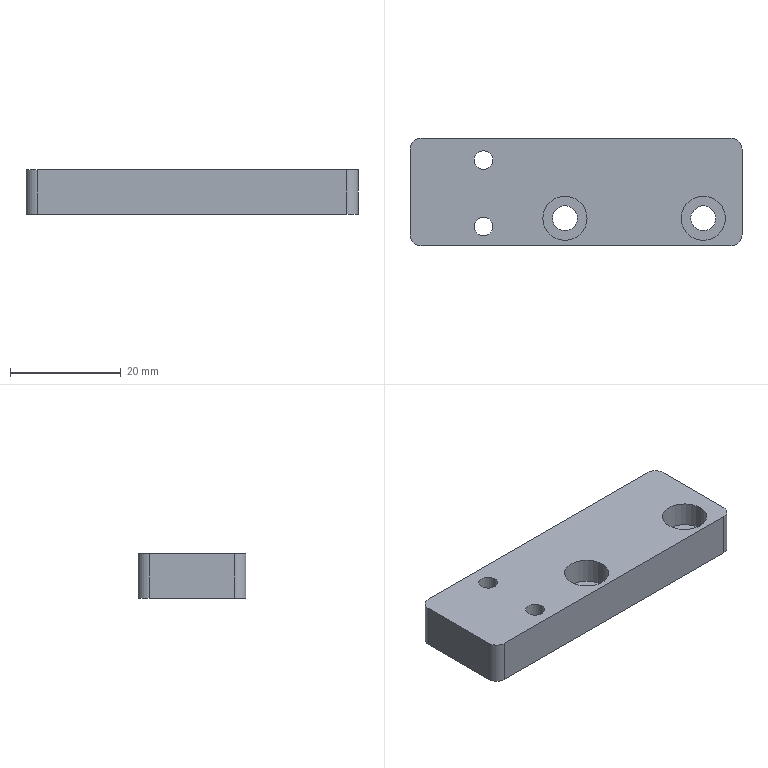Part | STEP file | FBDS-CS-001 | 1 solid | 30 faces | box 60 x 19.5 x 8 mm | volume 8486 mm3 | cylinder 20 | plane 10 | commonest cylinder face diameters 3.4 x4 4 x4 4.5 x4 6 x4 8 x4
STEP:
#1=CARTESIAN_POINT('',(16.3,15.5,3.4));
#2=VERTEX_POINT('',#1);
#3=CARTESIAN_POINT('',(10.3,15.5,3.4));
#4=VERTEX_POINT('',#3);
#5=CARTESIAN_POINT('',(13.3,15.5,3.4));
#6=DIRECTION('',(0.,0.,-1.));
#7=DIRECTION('',(-1.,0.,0.));
#8=AXIS2_PLACEMENT_3D('',#5,#6,#7);
#9=CIRCLE('',#8,3.);
#10=EDGE_CURVE('',#2,#4,#9,.T.);
#11=ORIENTED_EDGE('',*,*,#10,.F.);
#12=CARTESIAN_POINT('',(16.3,15.5,0.));
#13=VERTEX_POINT('',#12);
#14=CARTESIAN_POINT('',(16.3,15.5,0.));
#15=DIRECTION('',(0.,0.,-1.));
#16=VECTOR('',#15,1000.);
#17=LINE('',#14,#16);
#18=EDGE_CURVE('',#2,#13,#17,.T.);
#19=ORIENTED_EDGE('',*,*,#18,.T.);
#20=CARTESIAN_POINT('',(10.3,15.5,0.));
#21=VERTEX_POINT('',#20);
#22=CARTESIAN_POINT('',(13.3,15.5,0.));
#23=DIRECTION('',(0.,0.,-1.));
#24=DIRECTION('',(-1.,0.,0.));
#25=AXIS2_PLACEMENT_3D('',#22,#23,#24);
#26=CIRCLE('',#25,3.);
#27=EDGE_CURVE('',#13,#21,#26,.T.);
#28=ORIENTED_EDGE('',*,*,#27,.T.);
#29=CARTESIAN_POINT('',(10.3,15.5,0.));
#30=DIRECTION('',(0.,0.,-1.));
#31=VECTOR('',#30,1000.);
#32=LINE('',#29,#31);
#33=EDGE_CURVE('',#4,#21,#32,.T.);
#34=ORIENTED_EDGE('',*,*,#33,.F.);
#35=EDGE_LOOP('',(#11,#19,#28,#34));
#36=FACE_OUTER_BOUND('',#35,.T.);
#37=CARTESIAN_POINT('',(13.3,15.5,0.));
#38=DIRECTION('',(0.,0.,-1.));
#39=DIRECTION('',(-1.,0.,0.));
#40=AXIS2_PLACEMENT_3D('',#37,#38,#39);
#41=CYLINDRICAL_SURFACE('',#40,3.);
#42=ADVANCED_FACE('',(#36),#41,.F.);
#43=CARTESIAN_POINT('',(15.,15.5,8.));
#44=VERTEX_POINT('',#43);
#45=CARTESIAN_POINT('',(11.6,15.5,8.));
#46=VERTEX_POINT('',#45);
#47=CARTESIAN_POINT('',(13.3,15.5,8.));
#48=DIRECTION('',(0.,0.,-1.));
#49=DIRECTION('',(-1.,0.,0.));
#50=AXIS2_PLACEMENT_3D('',#47,#48,#49);
#51=CIRCLE('',#50,1.7);
#52=EDGE_CURVE('',#44,#46,#51,.T.);
#53=ORIENTED_EDGE('',*,*,#52,.F.);
#54=CARTESIAN_POINT('',(15.,15.5,3.4));
#55=VERTEX_POINT('',#54);
#56=CARTESIAN_POINT('',(15.,15.5,0.));
#57=DIRECTION('',(0.,0.,-1.));
#58=VECTOR('',#57,1000.);
#59=LINE('',#56,#58);
#60=EDGE_CURVE('',#44,#55,#59,.T.);
#61=ORIENTED_EDGE('',*,*,#60,.T.);
#62=CARTESIAN_POINT('',(11.6,15.5,3.4));
#63=VERTEX_POINT('',#62);
#64=CARTESIAN_POINT('',(13.3,15.5,3.4));
#65=DIRECTION('',(0.,0.,-1.));
#66=DIRECTION('',(-1.,0.,0.));
#67=AXIS2_PLACEMENT_3D('',#64,#65,#66);
#68=CIRCLE('',#67,1.7);
#69=EDGE_CURVE('',#55,#63,#68,.T.);
#70=ORIENTED_EDGE('',*,*,#69,.T.);
#71=CARTESIAN_POINT('',(11.6,15.5,0.));
#72=DIRECTION('',(0.,0.,-1.));
#73=VECTOR('',#72,1000.);
#74=LINE('',#71,#73);
#75=EDGE_CURVE('',#46,#63,#74,.T.);
#76=ORIENTED_EDGE('',*,*,#75,.F.);
#77=EDGE_LOOP('',(#53,#61,#70,#76));
#78=FACE_OUTER_BOUND('',#77,.T.);
#79=CARTESIAN_POINT('',(13.3,15.5,0.));
#80=DIRECTION('',(0.,0.,-1.));
#81=DIRECTION('',(-1.,0.,0.));
#82=AXIS2_PLACEMENT_3D('',#79,#80,#81);
#83=CYLINDRICAL_SURFACE('',#82,1.7);
#84=ADVANCED_FACE('',(#78),#83,.F.);
#85=CARTESIAN_POINT('',(16.3,3.5,3.4));
#86=VERTEX_POINT('',#85);
#87=CARTESIAN_POINT('',(10.3,3.5,3.4));
#88=VERTEX_POINT('',#87);
#89=CARTESIAN_POINT('',(13.3,3.5,3.4));
#90=DIRECTION('',(0.,0.,-1.));
#91=DIRECTION('',(-1.,0.,0.));
#92=AXIS2_PLACEMENT_3D('',#89,#90,#91);
#93=CIRCLE('',#92,3.);
#94=EDGE_CURVE('',#86,#88,#93,.T.);
#95=ORIENTED_EDGE('',*,*,#94,.F.);
#96=CARTESIAN_POINT('',(16.3,3.5,0.));
#97=VERTEX_POINT('',#96);
#98=CARTESIAN_POINT('',(16.3,3.5,0.));
#99=DIRECTION('',(0.,0.,-1.));
#100=VECTOR('',#99,1000.);
#101=LINE('',#98,#100);
#102=EDGE_CURVE('',#86,#97,#101,.T.);
#103=ORIENTED_EDGE('',*,*,#102,.T.);
#104=CARTESIAN_POINT('',(10.3,3.5,0.));
#105=VERTEX_POINT('',#104);
#106=CARTESIAN_POINT('',(13.3,3.5,0.));
#107=DIRECTION('',(0.,0.,-1.));
#108=DIRECTION('',(-1.,0.,0.));
#109=AXIS2_PLACEMENT_3D('',#106,#107,#108);
#110=CIRCLE('',#109,3.);
#111=EDGE_CURVE('',#97,#105,#110,.T.);
#112=ORIENTED_EDGE('',*,*,#111,.T.);
#113=CARTESIAN_POINT('',(10.3,3.5,0.));
#114=DIRECTION('',(0.,0.,-1.));
#115=VECTOR('',#114,1000.);
#116=LINE('',#113,#115);
#117=EDGE_CURVE('',#88,#105,#116,.T.);
#118=ORIENTED_EDGE('',*,*,#117,.F.);
#119=EDGE_LOOP('',(#95,#103,#112,#118));
#120=FACE_OUTER_BOUND('',#119,.T.);
#121=CARTESIAN_POINT('',(13.3,3.5,0.));
#122=DIRECTION('',(0.,0.,-1.));
#123=DIRECTION('',(-1.,0.,0.));
#124=AXIS2_PLACEMENT_3D('',#121,#122,#123);
#125=CYLINDRICAL_SURFACE('',#124,3.);
#126=ADVANCED_FACE('',(#120),#125,.F.);
#127=CARTESIAN_POINT('',(15.,3.5,8.));
#128=VERTEX_POINT('',#127);
#129=CARTESIAN_POINT('',(11.6,3.5,8.));
#130=VERTEX_POINT('',#129);
#131=CARTESIAN_POINT('',(13.3,3.5,8.));
#132=DIRECTION('',(0.,0.,-1.));
#133=DIRECTION('',(-1.,0.,0.));
#134=AXIS2_PLACEMENT_3D('',#131,#132,#133);
#135=CIRCLE('',#134,1.7);
#136=EDGE_CURVE('',#128,#130,#135,.T.);
#137=ORIENTED_EDGE('',*,*,#136,.F.);
#138=CARTESIAN_POINT('',(15.,3.5,3.4));
#139=VERTEX_POINT('',#138);
#140=CARTESIAN_POINT('',(15.,3.5,0.));
#141=DIRECTION('',(0.,0.,-1.));
#142=VECTOR('',#141,1000.);
#143=LINE('',#140,#142);
#144=EDGE_CURVE('',#128,#139,#143,.T.);
#145=ORIENTED_EDGE('',*,*,#144,.T.);
#146=CARTESIAN_POINT('',(11.6,3.5,3.4));
#147=VERTEX_POINT('',#146);
#148=CARTESIAN_POINT('',(13.3,3.5,3.4));
#149=DIRECTION('',(0.,0.,-1.));
#150=DIRECTION('',(-1.,0.,0.));
#151=AXIS2_PLACEMENT_3D('',#148,#149,#150);
#152=CIRCLE('',#151,1.7);
#153=EDGE_CURVE('',#139,#147,#152,.T.);
#154=ORIENTED_EDGE('',*,*,#153,.T.);
#155=CARTESIAN_POINT('',(11.6,3.5,0.));
#156=DIRECTION('',(0.,0.,-1.));
#157=VECTOR('',#156,1000.);
#158=LINE('',#155,#157);
#159=EDGE_CURVE('',#130,#147,#158,.T.);
#160=ORIENTED_EDGE('',*,*,#159,.F.);
#161=EDGE_LOOP('',(#137,#145,#154,#160));
#162=FACE_OUTER_BOUND('',#161,.T.);
#163=CARTESIAN_POINT('',(13.3,3.5,0.));
#164=DIRECTION('',(0.,0.,-1.));
#165=DIRECTION('',(-1.,0.,0.));
#166=AXIS2_PLACEMENT_3D('',#163,#164,#165);
#167=CYLINDRICAL_SURFACE('',#166,1.7);
#168=ADVANCED_FACE('',(#162),#167,.F.);
#169=CARTESIAN_POINT('',(24.,5.,3.4));
#170=VERTEX_POINT('',#169);
#171=CARTESIAN_POINT('',(32.,5.,3.4));
#172=VERTEX_POINT('',#171);
#173=CARTESIAN_POINT('',(28.,5.,3.4));
#174=DIRECTION('',(0.,0.,1.));
#175=DIRECTION('',(1.,0.,0.));
#176=AXIS2_PLACEMENT_3D('',#173,#174,#175);
#177=CIRCLE('',#176,4.);
#178=EDGE_CURVE('',#170,#172,#177,.T.);
#179=ORIENTED_EDGE('',*,*,#178,.F.);
#180=CARTESIAN_POINT('',(24.,5.,8.));
#181=VERTEX_POINT('',#180);
#182=CARTESIAN_POINT('',(24.,5.,8.));
#183=DIRECTION('',(0.,0.,1.));
#184=VECTOR('',#183,1000.);
#185=LINE('',#182,#184);
#186=EDGE_CURVE('',#170,#181,#185,.T.);
#187=ORIENTED_EDGE('',*,*,#186,.T.);
#188=CARTESIAN_POINT('',(32.,5.,8.));
#189=VERTEX_POINT('',#188);
#190=CARTESIAN_POINT('',(28.,5.,8.));
#191=DIRECTION('',(0.,0.,1.));
#192=DIRECTION('',(1.,0.,0.));
#193=AXIS2_PLACEMENT_3D('',#190,#191,#192);
#194=CIRCLE('',#193,4.);
#195=EDGE_CURVE('',#181,#189,#194,.T.);
#196=ORIENTED_EDGE('',*,*,#195,.T.);
#197=CARTESIAN_POINT('',(32.,5.,8.));
#198=DIRECTION('',(0.,0.,1.));
#199=VECTOR('',#198,1000.);
#200=LINE('',#197,#199);
#201=EDGE_CURVE('',#172,#189,#200,.T.);
#202=ORIENTED_EDGE('',*,*,#201,.F.);
#203=EDGE_LOOP('',(#179,#187,#196,#202));
#204=FACE_OUTER_BOUND('',#203,.T.);
#205=CARTESIAN_POINT('',(28.,5.,8.));
#206=DIRECTION('',(0.,0.,1.));
#207=DIRECTION('',(1.,0.,0.));
#208=AXIS2_PLACEMENT_3D('',#205,#206,#207);
#209=CYLINDRICAL_SURFACE('',#208,4.);
#210=ADVANCED_FACE('',(#204),#209,.F.);
#211=CARTESIAN_POINT('',(25.75,5.,0.));
#212=VERTEX_POINT('',#211);
#213=CARTESIAN_POINT('',(30.25,5.,0.));
#214=VERTEX_POINT('',#213);
#215=CARTESIAN_POINT('',(28.,5.,0.));
#216=DIRECTION('',(0.,0.,1.));
#217=DIRECTION('',(1.,0.,0.));
#218=AXIS2_PLACEMENT_3D('',#215,#216,#217);
#219=CIRCLE('',#218,2.25);
#220=EDGE_CURVE('',#212,#214,#219,.T.);
#221=ORIENTED_EDGE('',*,*,#220,.F.);
#222=CARTESIAN_POINT('',(25.75,5.,3.4));
#223=VERTEX_POINT('',#222);
#224=CARTESIAN_POINT('',(25.75,5.,8.));
#225=DIRECTION('',(0.,0.,1.));
#226=VECTOR('',#225,1000.);
#227=LINE('',#224,#226);
#228=EDGE_CURVE('',#212,#223,#227,.T.);
#229=ORIENTED_EDGE('',*,*,#228,.T.);
#230=CARTESIAN_POINT('',(30.25,5.,3.4));
#231=VERTEX_POINT('',#230);
#232=CARTESIAN_POINT('',(28.,5.,3.4));
#233=DIRECTION('',(0.,0.,1.));
#234=DIRECTION('',(1.,0.,0.));
#235=AXIS2_PLACEMENT_3D('',#232,#233,#234);
#236=CIRCLE('',#235,2.25);
#237=EDGE_CURVE('',#223,#231,#236,.T.);
#238=ORIENTED_EDGE('',*,*,#237,.T.);
#239=CARTESIAN_POINT('',(30.25,5.,8.));
#240=DIRECTION('',(0.,0.,1.));
#241=VECTOR('',#240,1000.);
#242=LINE('',#239,#241);
#243=EDGE_CURVE('',#214,#231,#242,.T.);
#244=ORIENTED_EDGE('',*,*,#243,.F.);
#245=EDGE_LOOP('',(#221,#229,#238,#244));
#246=FACE_OUTER_BOUND('',#245,.T.);
#247=CARTESIAN_POINT('',(28.,5.,8.));
#248=DIRECTION('',(0.,0.,1.));
#249=DIRECTION('',(1.,0.,0.));
#250=AXIS2_PLACEMENT_3D('',#247,#248,#249);
#251=CYLINDRICAL_SURFACE('',#250,2.25);
#252=ADVANCED_FACE('',(#246),#251,.F.);
#253=CARTESIAN_POINT('',(49.,5.,3.4));
#254=VERTEX_POINT('',#253);
#255=CARTESIAN_POINT('',(57.,5.,3.4));
#256=VERTEX_POINT('',#255);
#257=CARTESIAN_POINT('',(53.,5.,3.4));
#258=DIRECTION('',(0.,0.,1.));
#259=DIRECTION('',(1.,0.,0.));
#260=AXIS2_PLACEMENT_3D('',#257,#258,#259);
#261=CIRCLE('',#260,4.);
#262=EDGE_CURVE('',#254,#256,#261,.T.);
#263=ORIENTED_EDGE('',*,*,#262,.F.);
#264=CARTESIAN_POINT('',(49.,5.,8.));
#265=VERTEX_POINT('',#264);
#266=CARTESIAN_POINT('',(49.,5.,8.));
#267=DIRECTION('',(0.,0.,1.));
#268=VECTOR('',#267,1000.);
#269=LINE('',#266,#268);
#270=EDGE_CURVE('',#254,#265,#269,.T.);
#271=ORIENTED_EDGE('',*,*,#270,.T.);
#272=CARTESIAN_POINT('',(57.,5.,8.));
#273=VERTEX_POINT('',#272);
#274=CARTESIAN_POINT('',(53.,5.,8.));
#275=DIRECTION('',(0.,0.,1.));
#276=DIRECTION('',(1.,0.,0.));
#277=AXIS2_PLACEMENT_3D('',#274,#275,#276);
#278=CIRCLE('',#277,4.);
#279=EDGE_CURVE('',#265,#273,#278,.T.);
#280=ORIENTED_EDGE('',*,*,#279,.T.);
#281=CARTESIAN_POINT('',(57.,5.,8.));
#282=DIRECTION('',(0.,0.,1.));
#283=VECTOR('',#282,1000.);
#284=LINE('',#281,#283);
#285=EDGE_CURVE('',#256,#273,#284,.T.);
#286=ORIENTED_EDGE('',*,*,#285,.F.);
#287=EDGE_LOOP('',(#263,#271,#280,#286));
#288=FACE_OUTER_BOUND('',#287,.T.);
#289=CARTESIAN_POINT('',(53.,5.,8.));
#290=DIRECTION('',(0.,0.,1.));
#291=DIRECTION('',(1.,0.,0.));
#292=AXIS2_PLACEMENT_3D('',#289,#290,#291);
#293=CYLINDRICAL_SURFACE('',#292,4.);
#294=ADVANCED_FACE('',(#288),#293,.F.);
#295=CARTESIAN_POINT('',(50.75,5.,0.));
#296=VERTEX_POINT('',#295);
#297=CARTESIAN_POINT('',(55.25,5.,0.));
#298=VERTEX_POINT('',#297);
#299=CARTESIAN_POINT('',(53.,5.,0.));
#300=DIRECTION('',(0.,0.,1.));
#301=DIRECTION('',(1.,0.,0.));
#302=AXIS2_PLACEMENT_3D('',#299,#300,#301);
#303=CIRCLE('',#302,2.25);
#304=EDGE_CURVE('',#296,#298,#303,.T.);
#305=ORIENTED_EDGE('',*,*,#304,.F.);
#306=CARTESIAN_POINT('',(50.75,5.,3.4));
#307=VERTEX_POINT('',#306);
#308=CARTESIAN_POINT('',(50.75,5.,8.));
#309=DIRECTION('',(0.,0.,1.));
#310=VECTOR('',#309,1000.);
#311=LINE('',#308,#310);
#312=EDGE_CURVE('',#296,#307,#311,.T.);
#313=ORIENTED_EDGE('',*,*,#312,.T.);
#314=CARTESIAN_POINT('',(55.25,5.,3.4));
#315=VERTEX_POINT('',#314);
#316=CARTESIAN_POINT('',(53.,5.,3.4));
#317=DIRECTION('',(0.,0.,1.));
#318=DIRECTION('',(1.,0.,0.));
#319=AXIS2_PLACEMENT_3D('',#316,#317,#318);
#320=CIRCLE('',#319,2.25);
#321=EDGE_CURVE('',#307,#315,#320,.T.);
#322=ORIENTED_EDGE('',*,*,#321,.T.);
#323=CARTESIAN_POINT('',(55.25,5.,8.));
#324=DIRECTION('',(0.,0.,1.));
#325=VECTOR('',#324,1000.);
#326=LINE('',#323,#325);
#327=EDGE_CURVE('',#298,#315,#326,.T.);
#328=ORIENTED_EDGE('',*,*,#327,.F.);
#329=EDGE_LOOP('',(#305,#313,#322,#328));
#330=FACE_OUTER_BOUND('',#329,.T.);
#331=CARTESIAN_POINT('',(53.,5.,8.));
#332=DIRECTION('',(0.,0.,1.));
#333=DIRECTION('',(1.,0.,0.));
#334=AXIS2_PLACEMENT_3D('',#331,#332,#333);
#335=CYLINDRICAL_SURFACE('',#334,2.25);
#336=ADVANCED_FACE('',(#330),#335,.F.);
#337=CARTESIAN_POINT('',(0.,17.5,0.));
#338=VERTEX_POINT('',#337);
#339=CARTESIAN_POINT('',(0.,2.,0.));
#340=VERTEX_POINT('',#339);
#341=CARTESIAN_POINT('',(0.,0.,0.));
#342=DIRECTION('',(0.,-1.,0.));
#343=VECTOR('',#342,1000.);
#344=LINE('',#341,#343);
#345=EDGE_CURVE('',#338,#340,#344,.T.);
#346=ORIENTED_EDGE('',*,*,#345,.T.);
#347=CARTESIAN_POINT('',(0.,2.,8.));
#348=VERTEX_POINT('',#347);
#349=CARTESIAN_POINT('',(0.,2.,8.));
#350=DIRECTION('',(0.,0.,1.));
#351=VECTOR('',#350,1000.);
#352=LINE('',#349,#351);
#353=EDGE_CURVE('',#340,#348,#352,.T.);
#354=ORIENTED_EDGE('',*,*,#353,.T.);
#355=CARTESIAN_POINT('',(0.,17.5,8.));
#356=VERTEX_POINT('',#355);
#357=CARTESIAN_POINT('',(0.,0.,8.));
#358=DIRECTION('',(0.,-1.,0.));
#359=VECTOR('',#358,1000.);
#360=LINE('',#357,#359);
#361=EDGE_CURVE('',#356,#348,#360,.T.);
#362=ORIENTED_EDGE('',*,*,#361,.F.);
#363=CARTESIAN_POINT('',(0.,17.5,8.));
#364=DIRECTION('',(0.,0.,-1.));
#365=VECTOR('',#364,1000.);
#366=LINE('',#363,#365);
#367=EDGE_CURVE('',#356,#338,#366,.T.);
#368=ORIENTED_EDGE('',*,*,#367,.T.);
#369=EDGE_LOOP('',(#346,#354,#362,#368));
#370=FACE_OUTER_BOUND('',#369,.T.);
#371=CARTESIAN_POINT('',(0.,0.,8.));
#372=DIRECTION('',(1.,0.,0.));
#373=DIRECTION('',(0.,0.,-1.));
#374=AXIS2_PLACEMENT_3D('',#371,#372,#373);
#375=PLANE('',#374);
#376=ADVANCED_FACE('',(#370),#375,.F.);
#377=CARTESIAN_POINT('',(2.,0.,0.));
#378=VERTEX_POINT('',#377);
#379=CARTESIAN_POINT('',(58.,0.,0.));
#380=VERTEX_POINT('',#379);
#381=CARTESIAN_POINT('',(0.,0.,0.));
#382=DIRECTION('',(1.,0.,0.));
#383=VECTOR('',#382,1000.);
#384=LINE('',#381,#383);
#385=EDGE_CURVE('',#378,#380,#384,.T.);
#386=ORIENTED_EDGE('',*,*,#385,.T.);
#387=CARTESIAN_POINT('',(58.,0.,8.));
#388=VERTEX_POINT('',#387);
#389=CARTESIAN_POINT('',(58.,0.,8.));
#390=DIRECTION('',(0.,0.,1.));
#391=VECTOR('',#390,1000.);
#392=LINE('',#389,#391);
#393=EDGE_CURVE('',#380,#388,#392,.T.);
#394=ORIENTED_EDGE('',*,*,#393,.T.);
#395=CARTESIAN_POINT('',(2.,0.,8.));
#396=VERTEX_POINT('',#395);
#397=CARTESIAN_POINT('',(0.,0.,8.));
#398=DIRECTION('',(1.,0.,0.));
#399=VECTOR('',#398,1000.);
#400=LINE('',#397,#399);
#401=EDGE_CURVE('',#396,#388,#400,.T.);
#402=ORIENTED_EDGE('',*,*,#401,.F.);
#403=CARTESIAN_POINT('',(2.,0.,8.));
#404=DIRECTION('',(0.,0.,-1.));
#405=VECTOR('',#404,1000.);
#406=LINE('',#403,#405);
#407=EDGE_CURVE('',#396,#378,#406,.T.);
#408=ORIENTED_EDGE('',*,*,#407,.T.);
#409=EDGE_LOOP('',(#386,#394,#402,#408));
#410=FACE_OUTER_BOUND('',#409,.T.);
#411=CARTESIAN_POINT('',(0.,0.,8.));
#412=DIRECTION('',(0.,1.,0.));
#413=DIRECTION('',(0.,0.,1.));
#414=AXIS2_PLACEMENT_3D('',#411,#412,#413);
#415=PLANE('',#414);
#416=ADVANCED_FACE('',(#410),#415,.F.);
#417=CARTESIAN_POINT('',(60.,2.,8.));
#418=VERTEX_POINT('',#417);
#419=CARTESIAN_POINT('',(60.,17.5,8.));
#420=VERTEX_POINT('',#419);
#421=CARTESIAN_POINT('',(60.,0.,8.));
#422=DIRECTION('',(0.,1.,0.));
#423=VECTOR('',#422,1000.);
#424=LINE('',#421,#423);
#425=EDGE_CURVE('',#418,#420,#424,.T.);
#426=ORIENTED_EDGE('',*,*,#425,.F.);
#427=CARTESIAN_POINT('',(60.,2.,0.));
#428=VERTEX_POINT('',#427);
#429=CARTESIAN_POINT('',(60.,2.,8.));
#430=DIRECTION('',(0.,0.,-1.));
#431=VECTOR('',#430,1000.);
#432=LINE('',#429,#431);
#433=EDGE_CURVE('',#418,#428,#432,.T.);
#434=ORIENTED_EDGE('',*,*,#433,.T.);
#435=CARTESIAN_POINT('',(60.,17.5,0.));
#436=VERTEX_POINT('',#435);
#437=CARTESIAN_POINT('',(60.,0.,0.));
#438=DIRECTION('',(0.,1.,0.));
#439=VECTOR('',#438,1000.);
#440=LINE('',#437,#439);
#441=EDGE_CURVE('',#428,#436,#440,.T.);
#442=ORIENTED_EDGE('',*,*,#441,.T.);
#443=CARTESIAN_POINT('',(60.,17.5,8.));
#444=DIRECTION('',(0.,0.,1.));
#445=VECTOR('',#444,1000.);
#446=LINE('',#443,#445);
#447=EDGE_CURVE('',#436,#420,#446,.T.);
#448=ORIENTED_EDGE('',*,*,#447,.T.);
#449=EDGE_LOOP('',(#426,#434,#442,#448));
#450=FACE_OUTER_BOUND('',#449,.T.);
#451=CARTESIAN_POINT('',(60.,0.,8.));
#452=DIRECTION('',(-1.,0.,0.));
#453=DIRECTION('',(0.,0.,1.));
#454=AXIS2_PLACEMENT_3D('',#451,#452,#453);
#455=PLANE('',#454);
#456=ADVANCED_FACE('',(#450),#455,.F.);
#457=CARTESIAN_POINT('',(58.,19.5,8.));
#458=VERTEX_POINT('',#457);
#459=CARTESIAN_POINT('',(2.,19.5,8.));
#460=VERTEX_POINT('',#459);
#461=CARTESIAN_POINT('',(0.,19.5,8.));
#462=DIRECTION('',(-1.,0.,0.));
#463=VECTOR('',#462,1000.);
#464=LINE('',#461,#463);
#465=EDGE_CURVE('',#458,#460,#464,.T.);
#466=ORIENTED_EDGE('',*,*,#465,.F.);
#467=CARTESIAN_POINT('',(58.,19.5,0.));
#468=VERTEX_POINT('',#467);
#469=CARTESIAN_POINT('',(58.,19.5,8.));
#470=DIRECTION('',(0.,0.,-1.));
#471=VECTOR('',#470,1000.);
#472=LINE('',#469,#471);
#473=EDGE_CURVE('',#458,#468,#472,.T.);
#474=ORIENTED_EDGE('',*,*,#473,.T.);
#475=CARTESIAN_POINT('',(2.,19.5,0.));
#476=VERTEX_POINT('',#475);
#477=CARTESIAN_POINT('',(0.,19.5,0.));
#478=DIRECTION('',(-1.,0.,0.));
#479=VECTOR('',#478,1000.);
#480=LINE('',#477,#479);
#481=EDGE_CURVE('',#468,#476,#480,.T.);
#482=ORIENTED_EDGE('',*,*,#481,.T.);
#483=CARTESIAN_POINT('',(2.,19.5,8.));
#484=DIRECTION('',(0.,0.,1.));
#485=VECTOR('',#484,1000.);
#486=LINE('',#483,#485);
#487=EDGE_CURVE('',#476,#460,#486,.T.);
#488=ORIENTED_EDGE('',*,*,#487,.T.);
#489=EDGE_LOOP('',(#466,#474,#482,#488));
#490=FACE_OUTER_BOUND('',#489,.T.);
#491=CARTESIAN_POINT('',(0.,19.5,8.));
#492=DIRECTION('',(0.,-1.,0.));
#493=DIRECTION('',(0.,0.,-1.));
#494=AXIS2_PLACEMENT_3D('',#491,#492,#493);
#495=PLANE('',#494);
#496=ADVANCED_FACE('',(#490),#495,.F.);
#497=CARTESIAN_POINT('',(13.3,15.5,8.));
#498=DIRECTION('',(0.,0.,-1.));
#499=DIRECTION('',(-1.,0.,0.));
#500=AXIS2_PLACEMENT_3D('',#497,#498,#499);
#501=CIRCLE('',#500,1.7);
#502=EDGE_CURVE('',#46,#44,#501,.T.);
#503=ORIENTED_EDGE('',*,*,#502,.T.);
#504=ORIENTED_EDGE('',*,*,#52,.T.);
#505=EDGE_LOOP('',(#503,#504));
#506=FACE_BOUND('',#505,.T.);
#507=CARTESIAN_POINT('',(13.3,3.5,8.));
#508=DIRECTION('',(0.,0.,-1.));
#509=DIRECTION('',(-1.,0.,0.));
#510=AXIS2_PLACEMENT_3D('',#507,#508,#509);
#511=CIRCLE('',#510,1.7);
#512=EDGE_CURVE('',#130,#128,#511,.T.);
#513=ORIENTED_EDGE('',*,*,#512,.T.);
#514=ORIENTED_EDGE('',*,*,#136,.T.);
#515=EDGE_LOOP('',(#513,#514));
#516=FACE_BOUND('',#515,.T.);
#517=CARTESIAN_POINT('',(28.,5.,8.));
#518=DIRECTION('',(0.,0.,1.));
#519=DIRECTION('',(1.,0.,0.));
#520=AXIS2_PLACEMENT_3D('',#517,#518,#519);
#521=CIRCLE('',#520,4.);
#522=EDGE_CURVE('',#189,#181,#521,.T.);
#523=ORIENTED_EDGE('',*,*,#522,.F.);
#524=ORIENTED_EDGE('',*,*,#195,.F.);
#525=EDGE_LOOP('',(#523,#524));
#526=FACE_BOUND('',#525,.T.);
#527=CARTESIAN_POINT('',(53.,5.,8.));
#528=DIRECTION('',(0.,0.,1.));
#529=DIRECTION('',(1.,0.,0.));
#530=AXIS2_PLACEMENT_3D('',#527,#528,#529);
#531=CIRCLE('',#530,4.);
#532=EDGE_CURVE('',#273,#265,#531,.T.);
#533=ORIENTED_EDGE('',*,*,#532,.F.);
#534=ORIENTED_EDGE('',*,*,#279,.F.);
#535=EDGE_LOOP('',(#533,#534));
#536=FACE_BOUND('',#535,.T.);
#537=ORIENTED_EDGE('',*,*,#401,.T.);
#538=CARTESIAN_POINT('',(58.,2.,8.));
#539=DIRECTION('',(0.,0.,1.));
#540=DIRECTION('',(-1.,0.,0.));
#541=AXIS2_PLACEMENT_3D('',#538,#539,#540);
#542=CIRCLE('',#541,2.);
#543=EDGE_CURVE('',#388,#418,#542,.T.);
#544=ORIENTED_EDGE('',*,*,#543,.T.);
#545=ORIENTED_EDGE('',*,*,#425,.T.);
#546=CARTESIAN_POINT('',(58.,17.5,8.));
#547=DIRECTION('',(0.,0.,1.));
#548=DIRECTION('',(-1.,0.,0.));
#549=AXIS2_PLACEMENT_3D('',#546,#547,#548);
#550=CIRCLE('',#549,2.);
#551=EDGE_CURVE('',#420,#458,#550,.T.);
#552=ORIENTED_EDGE('',*,*,#551,.T.);
#553=ORIENTED_EDGE('',*,*,#465,.T.);
#554=CARTESIAN_POINT('',(2.,17.5,8.));
#555=DIRECTION('',(0.,0.,1.));
#556=DIRECTION('',(-1.,0.,0.));
#557=AXIS2_PLACEMENT_3D('',#554,#555,#556);
#558=CIRCLE('',#557,2.);
#559=EDGE_CURVE('',#460,#356,#558,.T.);
#560=ORIENTED_EDGE('',*,*,#559,.T.);
#561=ORIENTED_EDGE('',*,*,#361,.T.);
#562=CARTESIAN_POINT('',(2.,2.,8.));
#563=DIRECTION('',(0.,0.,1.));
#564=DIRECTION('',(-1.,0.,0.));
#565=AXIS2_PLACEMENT_3D('',#562,#563,#564);
#566=CIRCLE('',#565,2.);
#567=EDGE_CURVE('',#348,#396,#566,.T.);
#568=ORIENTED_EDGE('',*,*,#567,.T.);
#569=EDGE_LOOP('',(#537,#544,#545,#552,#553,#560,#561,#568));
#570=FACE_OUTER_BOUND('',#569,.T.);
#571=CARTESIAN_POINT('',(0.,0.,8.));
#572=DIRECTION('',(0.,0.,-1.));
#573=DIRECTION('',(-1.,0.,0.));
#574=AXIS2_PLACEMENT_3D('',#571,#572,#573);
#575=PLANE('',#574);
#576=ADVANCED_FACE('',(#506,#516,#526,#536,#570),#575,.F.);
#577=CARTESIAN_POINT('',(13.3,15.5,0.));
#578=DIRECTION('',(0.,0.,-1.));
#579=DIRECTION('',(-1.,0.,0.));
#580=AXIS2_PLACEMENT_3D('',#577,#578,#579);
#581=CIRCLE('',#580,3.);
#582=EDGE_CURVE('',#21,#13,#581,.T.);
#583=ORIENTED_EDGE('',*,*,#582,.F.);
#584=ORIENTED_EDGE('',*,*,#27,.F.);
#585=EDGE_LOOP('',(#583,#584));
#586=FACE_BOUND('',#585,.T.);
#587=CARTESIAN_POINT('',(13.3,3.5,0.));
#588=DIRECTION('',(0.,0.,-1.));
#589=DIRECTION('',(-1.,0.,0.));
#590=AXIS2_PLACEMENT_3D('',#587,#588,#589);
#591=CIRCLE('',#590,3.);
#592=EDGE_CURVE('',#105,#97,#591,.T.);
#593=ORIENTED_EDGE('',*,*,#592,.F.);
#594=ORIENTED_EDGE('',*,*,#111,.F.);
#595=EDGE_LOOP('',(#593,#594));
#596=FACE_BOUND('',#595,.T.);
#597=CARTESIAN_POINT('',(28.,5.,0.));
#598=DIRECTION('',(0.,0.,1.));
#599=DIRECTION('',(1.,0.,0.));
#600=AXIS2_PLACEMENT_3D('',#597,#598,#599);
#601=CIRCLE('',#600,2.25);
#602=EDGE_CURVE('',#214,#212,#601,.T.);
#603=ORIENTED_EDGE('',*,*,#602,.T.);
#604=ORIENTED_EDGE('',*,*,#220,.T.);
#605=EDGE_LOOP('',(#603,#604));
#606=FACE_BOUND('',#605,.T.);
#607=CARTESIAN_POINT('',(53.,5.,0.));
#608=DIRECTION('',(0.,0.,1.));
#609=DIRECTION('',(1.,0.,0.));
#610=AXIS2_PLACEMENT_3D('',#607,#608,#609);
#611=CIRCLE('',#610,2.25);
#612=EDGE_CURVE('',#298,#296,#611,.T.);
#613=ORIENTED_EDGE('',*,*,#612,.T.);
#614=ORIENTED_EDGE('',*,*,#304,.T.);
#615=EDGE_LOOP('',(#613,#614));
#616=FACE_BOUND('',#615,.T.);
#617=ORIENTED_EDGE('',*,*,#441,.F.);
#618=CARTESIAN_POINT('',(58.,2.,0.));
#619=DIRECTION('',(0.,0.,-1.));
#620=DIRECTION('',(-1.,0.,0.));
#621=AXIS2_PLACEMENT_3D('',#618,#619,#620);
#622=CIRCLE('',#621,2.);
#623=EDGE_CURVE('',#428,#380,#622,.T.);
#624=ORIENTED_EDGE('',*,*,#623,.T.);
#625=ORIENTED_EDGE('',*,*,#385,.F.);
#626=CARTESIAN_POINT('',(2.,2.,0.));
#627=DIRECTION('',(0.,0.,-1.));
#628=DIRECTION('',(-1.,0.,0.));
#629=AXIS2_PLACEMENT_3D('',#626,#627,#628);
#630=CIRCLE('',#629,2.);
#631=EDGE_CURVE('',#378,#340,#630,.T.);
#632=ORIENTED_EDGE('',*,*,#631,.T.);
#633=ORIENTED_EDGE('',*,*,#345,.F.);
#634=CARTESIAN_POINT('',(2.,17.5,0.));
#635=DIRECTION('',(0.,0.,-1.));
#636=DIRECTION('',(-1.,0.,0.));
#637=AXIS2_PLACEMENT_3D('',#634,#635,#636);
#638=CIRCLE('',#637,2.);
#639=EDGE_CURVE('',#338,#476,#638,.T.);
#640=ORIENTED_EDGE('',*,*,#639,.T.);
#641=ORIENTED_EDGE('',*,*,#481,.F.);
#642=CARTESIAN_POINT('',(58.,17.5,0.));
#643=DIRECTION('',(0.,0.,-1.));
#644=DIRECTION('',(-1.,0.,0.));
#645=AXIS2_PLACEMENT_3D('',#642,#643,#644);
#646=CIRCLE('',#645,2.);
#647=EDGE_CURVE('',#468,#436,#646,.T.);
#648=ORIENTED_EDGE('',*,*,#647,.T.);
#649=EDGE_LOOP('',(#617,#624,#625,#632,#633,#640,#641,#648));
#650=FACE_OUTER_BOUND('',#649,.T.);
#651=CARTESIAN_POINT('',(0.,0.,0.));
#652=DIRECTION('',(0.,0.,-1.));
#653=DIRECTION('',(-1.,0.,0.));
#654=AXIS2_PLACEMENT_3D('',#651,#652,#653);
#655=PLANE('',#654);
#656=ADVANCED_FACE('',(#586,#596,#606,#616,#650),#655,.T.);
#657=ORIENTED_EDGE('',*,*,#312,.F.);
#658=ORIENTED_EDGE('',*,*,#612,.F.);
#659=ORIENTED_EDGE('',*,*,#327,.T.);
#660=CARTESIAN_POINT('',(53.,5.,3.4));
#661=DIRECTION('',(0.,0.,1.));
#662=DIRECTION('',(1.,0.,0.));
#663=AXIS2_PLACEMENT_3D('',#660,#661,#662);
#664=CIRCLE('',#663,2.25);
#665=EDGE_CURVE('',#315,#307,#664,.T.);
#666=ORIENTED_EDGE('',*,*,#665,.T.);
#667=EDGE_LOOP('',(#657,#658,#659,#666));
#668=FACE_OUTER_BOUND('',#667,.T.);
#669=CARTESIAN_POINT('',(53.,5.,8.));
#670=DIRECTION('',(0.,0.,1.));
#671=DIRECTION('',(1.,0.,0.));
#672=AXIS2_PLACEMENT_3D('',#669,#670,#671);
#673=CYLINDRICAL_SURFACE('',#672,2.25);
#674=ADVANCED_FACE('',(#668),#673,.F.);
#675=ORIENTED_EDGE('',*,*,#665,.F.);
#676=ORIENTED_EDGE('',*,*,#321,.F.);
#677=EDGE_LOOP('',(#675,#676));
#678=FACE_BOUND('',#677,.T.);
#679=CARTESIAN_POINT('',(53.,5.,3.4));
#680=DIRECTION('',(0.,0.,1.));
#681=DIRECTION('',(1.,0.,0.));
#682=AXIS2_PLACEMENT_3D('',#679,#680,#681);
#683=CIRCLE('',#682,4.);
#684=EDGE_CURVE('',#256,#254,#683,.T.);
#685=ORIENTED_EDGE('',*,*,#684,.T.);
#686=ORIENTED_EDGE('',*,*,#262,.T.);
#687=EDGE_LOOP('',(#685,#686));
#688=FACE_OUTER_BOUND('',#687,.T.);
#689=CARTESIAN_POINT('',(55.25,5.,3.4));
#690=DIRECTION('',(0.,0.,-1.));
#691=DIRECTION('',(-1.,0.,0.));
#692=AXIS2_PLACEMENT_3D('',#689,#690,#691);
#693=PLANE('',#692);
#694=ADVANCED_FACE('',(#678,#688),#693,.F.);
#695=ORIENTED_EDGE('',*,*,#270,.F.);
#696=ORIENTED_EDGE('',*,*,#684,.F.);
#697=ORIENTED_EDGE('',*,*,#285,.T.);
#698=ORIENTED_EDGE('',*,*,#532,.T.);
#699=EDGE_LOOP('',(#695,#696,#697,#698));
#700=FACE_OUTER_BOUND('',#699,.T.);
#701=CARTESIAN_POINT('',(53.,5.,8.));
#702=DIRECTION('',(0.,0.,1.));
#703=DIRECTION('',(1.,0.,0.));
#704=AXIS2_PLACEMENT_3D('',#701,#702,#703);
#705=CYLINDRICAL_SURFACE('',#704,4.);
#706=ADVANCED_FACE('',(#700),#705,.F.);
#707=ORIENTED_EDGE('',*,*,#228,.F.);
#708=ORIENTED_EDGE('',*,*,#602,.F.);
#709=ORIENTED_EDGE('',*,*,#243,.T.);
#710=CARTESIAN_POINT('',(28.,5.,3.4));
#711=DIRECTION('',(0.,0.,1.));
#712=DIRECTION('',(1.,0.,0.));
#713=AXIS2_PLACEMENT_3D('',#710,#711,#712);
#714=CIRCLE('',#713,2.25);
#715=EDGE_CURVE('',#231,#223,#714,.T.);
#716=ORIENTED_EDGE('',*,*,#715,.T.);
#717=EDGE_LOOP('',(#707,#708,#709,#716));
#718=FACE_OUTER_BOUND('',#717,.T.);
#719=CARTESIAN_POINT('',(28.,5.,8.));
#720=DIRECTION('',(0.,0.,1.));
#721=DIRECTION('',(1.,0.,0.));
#722=AXIS2_PLACEMENT_3D('',#719,#720,#721);
#723=CYLINDRICAL_SURFACE('',#722,2.25);
#724=ADVANCED_FACE('',(#718),#723,.F.);
#725=ORIENTED_EDGE('',*,*,#715,.F.);
#726=ORIENTED_EDGE('',*,*,#237,.F.);
#727=EDGE_LOOP('',(#725,#726));
#728=FACE_BOUND('',#727,.T.);
#729=CARTESIAN_POINT('',(28.,5.,3.4));
#730=DIRECTION('',(0.,0.,1.));
#731=DIRECTION('',(1.,0.,0.));
#732=AXIS2_PLACEMENT_3D('',#729,#730,#731);
#733=CIRCLE('',#732,4.);
#734=EDGE_CURVE('',#172,#170,#733,.T.);
#735=ORIENTED_EDGE('',*,*,#734,.T.);
#736=ORIENTED_EDGE('',*,*,#178,.T.);
#737=EDGE_LOOP('',(#735,#736));
#738=FACE_OUTER_BOUND('',#737,.T.);
#739=CARTESIAN_POINT('',(30.25,5.,3.4));
#740=DIRECTION('',(0.,0.,-1.));
#741=DIRECTION('',(-1.,0.,0.));
#742=AXIS2_PLACEMENT_3D('',#739,#740,#741);
#743=PLANE('',#742);
#744=ADVANCED_FACE('',(#728,#738),#743,.F.);
#745=ORIENTED_EDGE('',*,*,#186,.F.);
#746=ORIENTED_EDGE('',*,*,#734,.F.);
#747=ORIENTED_EDGE('',*,*,#201,.T.);
#748=ORIENTED_EDGE('',*,*,#522,.T.);
#749=EDGE_LOOP('',(#745,#746,#747,#748));
#750=FACE_OUTER_BOUND('',#749,.T.);
#751=CARTESIAN_POINT('',(28.,5.,8.));
#752=DIRECTION('',(0.,0.,1.));
#753=DIRECTION('',(1.,0.,0.));
#754=AXIS2_PLACEMENT_3D('',#751,#752,#753);
#755=CYLINDRICAL_SURFACE('',#754,4.);
#756=ADVANCED_FACE('',(#750),#755,.F.);
#757=ORIENTED_EDGE('',*,*,#144,.F.);
#758=ORIENTED_EDGE('',*,*,#512,.F.);
#759=ORIENTED_EDGE('',*,*,#159,.T.);
#760=CARTESIAN_POINT('',(13.3,3.5,3.4));
#761=DIRECTION('',(0.,0.,-1.));
#762=DIRECTION('',(-1.,0.,0.));
#763=AXIS2_PLACEMENT_3D('',#760,#761,#762);
#764=CIRCLE('',#763,1.7);
#765=EDGE_CURVE('',#147,#139,#764,.T.);
#766=ORIENTED_EDGE('',*,*,#765,.T.);
#767=EDGE_LOOP('',(#757,#758,#759,#766));
#768=FACE_OUTER_BOUND('',#767,.T.);
#769=CARTESIAN_POINT('',(13.3,3.5,0.));
#770=DIRECTION('',(0.,0.,-1.));
#771=DIRECTION('',(-1.,0.,0.));
#772=AXIS2_PLACEMENT_3D('',#769,#770,#771);
#773=CYLINDRICAL_SURFACE('',#772,1.7);
#774=ADVANCED_FACE('',(#768),#773,.F.);
#775=ORIENTED_EDGE('',*,*,#765,.F.);
#776=ORIENTED_EDGE('',*,*,#153,.F.);
#777=EDGE_LOOP('',(#775,#776));
#778=FACE_BOUND('',#777,.T.);
#779=CARTESIAN_POINT('',(13.3,3.5,3.4));
#780=DIRECTION('',(0.,0.,-1.));
#781=DIRECTION('',(-1.,0.,0.));
#782=AXIS2_PLACEMENT_3D('',#779,#780,#781);
#783=CIRCLE('',#782,3.);
#784=EDGE_CURVE('',#88,#86,#783,.T.);
#785=ORIENTED_EDGE('',*,*,#784,.T.);
#786=ORIENTED_EDGE('',*,*,#94,.T.);
#787=EDGE_LOOP('',(#785,#786));
#788=FACE_OUTER_BOUND('',#787,.T.);
#789=CARTESIAN_POINT('',(15.,3.5,3.4));
#790=DIRECTION('',(0.,0.,1.));
#791=DIRECTION('',(1.,0.,0.));
#792=AXIS2_PLACEMENT_3D('',#789,#790,#791);
#793=PLANE('',#792);
#794=ADVANCED_FACE('',(#778,#788),#793,.F.);
#795=ORIENTED_EDGE('',*,*,#102,.F.);
#796=ORIENTED_EDGE('',*,*,#784,.F.);
#797=ORIENTED_EDGE('',*,*,#117,.T.);
#798=ORIENTED_EDGE('',*,*,#592,.T.);
#799=EDGE_LOOP('',(#795,#796,#797,#798));
#800=FACE_OUTER_BOUND('',#799,.T.);
#801=CARTESIAN_POINT('',(13.3,3.5,0.));
#802=DIRECTION('',(0.,0.,-1.));
#803=DIRECTION('',(-1.,0.,0.));
#804=AXIS2_PLACEMENT_3D('',#801,#802,#803);
#805=CYLINDRICAL_SURFACE('',#804,3.);
#806=ADVANCED_FACE('',(#800),#805,.F.);
#807=ORIENTED_EDGE('',*,*,#60,.F.);
#808=ORIENTED_EDGE('',*,*,#502,.F.);
#809=ORIENTED_EDGE('',*,*,#75,.T.);
#810=CARTESIAN_POINT('',(13.3,15.5,3.4));
#811=DIRECTION('',(0.,0.,-1.));
#812=DIRECTION('',(-1.,0.,0.));
#813=AXIS2_PLACEMENT_3D('',#810,#811,#812);
#814=CIRCLE('',#813,1.7);
#815=EDGE_CURVE('',#63,#55,#814,.T.);
#816=ORIENTED_EDGE('',*,*,#815,.T.);
#817=EDGE_LOOP('',(#807,#808,#809,#816));
#818=FACE_OUTER_BOUND('',#817,.T.);
#819=CARTESIAN_POINT('',(13.3,15.5,0.));
#820=DIRECTION('',(0.,0.,-1.));
#821=DIRECTION('',(-1.,0.,0.));
#822=AXIS2_PLACEMENT_3D('',#819,#820,#821);
#823=CYLINDRICAL_SURFACE('',#822,1.7);
#824=ADVANCED_FACE('',(#818),#823,.F.);
#825=ORIENTED_EDGE('',*,*,#815,.F.);
#826=ORIENTED_EDGE('',*,*,#69,.F.);
#827=EDGE_LOOP('',(#825,#826));
#828=FACE_BOUND('',#827,.T.);
#829=CARTESIAN_POINT('',(13.3,15.5,3.4));
#830=DIRECTION('',(0.,0.,-1.));
#831=DIRECTION('',(-1.,0.,0.));
#832=AXIS2_PLACEMENT_3D('',#829,#830,#831);
#833=CIRCLE('',#832,3.);
#834=EDGE_CURVE('',#4,#2,#833,.T.);
#835=ORIENTED_EDGE('',*,*,#834,.T.);
#836=ORIENTED_EDGE('',*,*,#10,.T.);
#837=EDGE_LOOP('',(#835,#836));
#838=FACE_OUTER_BOUND('',#837,.T.);
#839=CARTESIAN_POINT('',(15.,15.5,3.4));
#840=DIRECTION('',(0.,0.,1.));
#841=DIRECTION('',(1.,0.,0.));
#842=AXIS2_PLACEMENT_3D('',#839,#840,#841);
#843=PLANE('',#842);
#844=ADVANCED_FACE('',(#828,#838),#843,.F.);
#845=ORIENTED_EDGE('',*,*,#18,.F.);
#846=ORIENTED_EDGE('',*,*,#834,.F.);
#847=ORIENTED_EDGE('',*,*,#33,.T.);
#848=ORIENTED_EDGE('',*,*,#582,.T.);
#849=EDGE_LOOP('',(#845,#846,#847,#848));
#850=FACE_OUTER_BOUND('',#849,.T.);
#851=CARTESIAN_POINT('',(13.3,15.5,0.));
#852=DIRECTION('',(0.,0.,-1.));
#853=DIRECTION('',(-1.,0.,0.));
#854=AXIS2_PLACEMENT_3D('',#851,#852,#853);
#855=CYLINDRICAL_SURFACE('',#854,3.);
#856=ADVANCED_FACE('',(#850),#855,.F.);
#857=ORIENTED_EDGE('',*,*,#543,.F.);
#858=ORIENTED_EDGE('',*,*,#393,.F.);
#859=ORIENTED_EDGE('',*,*,#623,.F.);
#860=ORIENTED_EDGE('',*,*,#433,.F.);
#861=EDGE_LOOP('',(#857,#858,#859,#860));
#862=FACE_OUTER_BOUND('',#861,.T.);
#863=CARTESIAN_POINT('',(58.,2.,8.));
#864=DIRECTION('',(0.,0.,-1.));
#865=DIRECTION('',(-1.,0.,0.));
#866=AXIS2_PLACEMENT_3D('',#863,#864,#865);
#867=CYLINDRICAL_SURFACE('',#866,2.);
#868=ADVANCED_FACE('',(#862),#867,.T.);
#869=ORIENTED_EDGE('',*,*,#551,.F.);
#870=ORIENTED_EDGE('',*,*,#447,.F.);
#871=ORIENTED_EDGE('',*,*,#647,.F.);
#872=ORIENTED_EDGE('',*,*,#473,.F.);
#873=EDGE_LOOP('',(#869,#870,#871,#872));
#874=FACE_OUTER_BOUND('',#873,.T.);
#875=CARTESIAN_POINT('',(58.,17.5,8.));
#876=DIRECTION('',(0.,0.,-1.));
#877=DIRECTION('',(-1.,0.,0.));
#878=AXIS2_PLACEMENT_3D('',#875,#876,#877);
#879=CYLINDRICAL_SURFACE('',#878,2.);
#880=ADVANCED_FACE('',(#874),#879,.T.);
#881=ORIENTED_EDGE('',*,*,#567,.F.);
#882=ORIENTED_EDGE('',*,*,#353,.F.);
#883=ORIENTED_EDGE('',*,*,#631,.F.);
#884=ORIENTED_EDGE('',*,*,#407,.F.);
#885=EDGE_LOOP('',(#881,#882,#883,#884));
#886=FACE_OUTER_BOUND('',#885,.T.);
#887=CARTESIAN_POINT('',(2.,2.,8.));
#888=DIRECTION('',(0.,0.,-1.));
#889=DIRECTION('',(-1.,0.,0.));
#890=AXIS2_PLACEMENT_3D('',#887,#888,#889);
#891=CYLINDRICAL_SURFACE('',#890,2.);
#892=ADVANCED_FACE('',(#886),#891,.T.);
#893=ORIENTED_EDGE('',*,*,#559,.F.);
#894=ORIENTED_EDGE('',*,*,#487,.F.);
#895=ORIENTED_EDGE('',*,*,#639,.F.);
#896=ORIENTED_EDGE('',*,*,#367,.F.);
#897=EDGE_LOOP('',(#893,#894,#895,#896));
#898=FACE_OUTER_BOUND('',#897,.T.);
#899=CARTESIAN_POINT('',(2.,17.5,8.));
#900=DIRECTION('',(0.,0.,-1.));
#901=DIRECTION('',(-1.,0.,0.));
#902=AXIS2_PLACEMENT_3D('',#899,#900,#901);
#903=CYLINDRICAL_SURFACE('',#902,2.);
#904=ADVANCED_FACE('',(#898),#903,.T.);
#905=CLOSED_SHELL('',(#42,#84,#126,#168,#210,#252,#294,#336,#376,#416,#456,#496,#576,#656,#674,#694,#706,#724,#744,#756,#774,#794,#806,#824,#844,#856,#868,#880,#892,#904));
#906=MANIFOLD_SOLID_BREP('',#905);
#907=CARTESIAN_POINT('',(0.,0.,0.));
#908=DIRECTION('',(0.,0.,1.));
#909=DIRECTION('',(1.,0.,0.));
#910=AXIS2_PLACEMENT_3D('',#907,#908,#909);
#911=(LENGTH_UNIT()NAMED_UNIT(*)SI_UNIT(.MILLI.,.METRE.));
#912=UNCERTAINTY_MEASURE_WITH_UNIT(LENGTH_MEASURE(0.00001),#911,'','');
#913=(NAMED_UNIT(*)PLANE_ANGLE_UNIT()SI_UNIT($,.RADIAN.));
#914=(NAMED_UNIT(*)SI_UNIT($,.STERADIAN.)SOLID_ANGLE_UNIT());
#915=(GEOMETRIC_REPRESENTATION_CONTEXT(3)GLOBAL_UNCERTAINTY_ASSIGNED_CONTEXT((#912))GLOBAL_UNIT_ASSIGNED_CONTEXT((#911,#913,#914))REPRESENTATION_CONTEXT('',''));
#916=ADVANCED_BREP_SHAPE_REPRESENTATION('',(#906,#910),#915);